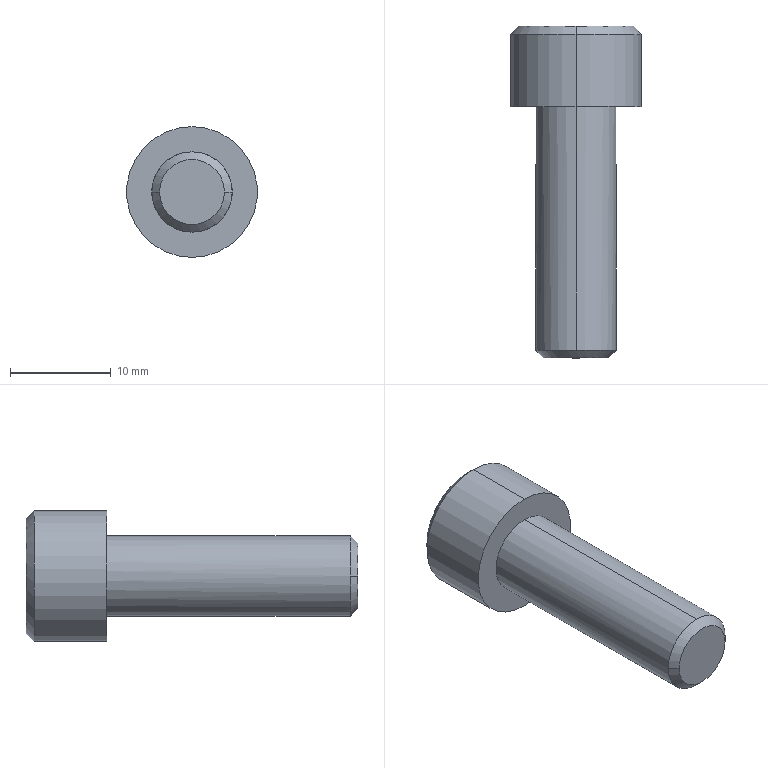Part | STEP file | PN59104-141_M_SHCSM8x1.25x25 | 1 solid | 18 faces | box 13 x 33 x 13 mm | volume 2174 mm3 | plane 10 | cylinder 4 | cone 4 | commonest cylinder face diameters 8 x2 13 x2
STEP:
#1=CARTESIAN_POINT('',(0.,0.,-4.));
#2=VERTEX_POINT('',#1);
#3=CARTESIAN_POINT('',(0.,0.,4.));
#4=VERTEX_POINT('',#3);
#5=CARTESIAN_POINT('',(0.,0.,0.));
#6=DIRECTION('',(0.,-1.,0.));
#7=DIRECTION('',(0.,0.,-1.));
#8=AXIS2_PLACEMENT_3D('',#5,#6,#7);
#9=CIRCLE('',#8,4.);
#10=EDGE_CURVE('',#2,#4,#9,.T.);
#11=ORIENTED_EDGE('',*,*,#10,.T.);
#12=CARTESIAN_POINT('',(0.,-24.233,4.));
#13=VERTEX_POINT('',#12);
#14=CARTESIAN_POINT('',(0.,-25.,4.));
#15=DIRECTION('',(0.,-1.,0.));
#16=VECTOR('',#15,1000.);
#17=LINE('',#14,#16);
#18=EDGE_CURVE('',#4,#13,#17,.T.);
#19=ORIENTED_EDGE('',*,*,#18,.T.);
#20=CARTESIAN_POINT('',(4.,-24.233,0.));
#21=VERTEX_POINT('',#20);
#22=CARTESIAN_POINT('',(0.,-24.233,0.));
#23=DIRECTION('',(0.,1.,0.));
#24=DIRECTION('',(0.,0.,-1.));
#25=AXIS2_PLACEMENT_3D('',#22,#23,#24);
#26=CIRCLE('',#25,4.);
#27=EDGE_CURVE('',#13,#21,#26,.T.);
#28=ORIENTED_EDGE('',*,*,#27,.T.);
#29=CARTESIAN_POINT('',(0.,-24.233,-4.));
#30=VERTEX_POINT('',#29);
#31=CARTESIAN_POINT('',(0.,-24.233,0.));
#32=DIRECTION('',(0.,1.,0.));
#33=DIRECTION('',(0.,0.,-1.));
#34=AXIS2_PLACEMENT_3D('',#31,#32,#33);
#35=CIRCLE('',#34,4.);
#36=EDGE_CURVE('',#21,#30,#35,.T.);
#37=ORIENTED_EDGE('',*,*,#36,.T.);
#38=CARTESIAN_POINT('',(0.,-25.,-4.));
#39=DIRECTION('',(0.,-1.,0.));
#40=VECTOR('',#39,1000.);
#41=LINE('',#38,#40);
#42=EDGE_CURVE('',#2,#30,#41,.T.);
#43=ORIENTED_EDGE('',*,*,#42,.F.);
#44=EDGE_LOOP('',(#11,#19,#28,#37,#43));
#45=FACE_OUTER_BOUND('',#44,.T.);
#46=CARTESIAN_POINT('',(0.,-25.,0.));
#47=DIRECTION('',(0.,-1.,0.));
#48=DIRECTION('',(0.,0.,-1.));
#49=AXIS2_PLACEMENT_3D('',#46,#47,#48);
#50=CYLINDRICAL_SURFACE('',#49,4.);
#51=ADVANCED_FACE('',(#45),#50,.T.);
#52=CARTESIAN_POINT('',(-3.233,-25.,0.));
#53=VERTEX_POINT('',#52);
#54=CARTESIAN_POINT('',(3.233,-25.,0.));
#55=VERTEX_POINT('',#54);
#56=CARTESIAN_POINT('',(0.,-25.,0.));
#57=DIRECTION('',(0.,1.,0.));
#58=DIRECTION('',(-1.,0.,0.));
#59=AXIS2_PLACEMENT_3D('',#56,#57,#58);
#60=CIRCLE('',#59,3.233);
#61=EDGE_CURVE('',#53,#55,#60,.T.);
#62=ORIENTED_EDGE('',*,*,#61,.T.);
#63=CARTESIAN_POINT('',(4.,-24.233,0.));
#64=DIRECTION('',(0.7071,0.7071,0.));
#65=VECTOR('',#64,1000.);
#66=LINE('',#63,#65);
#67=EDGE_CURVE('',#55,#21,#66,.T.);
#68=ORIENTED_EDGE('',*,*,#67,.T.);
#69=ORIENTED_EDGE('',*,*,#27,.F.);
#70=CARTESIAN_POINT('',(-4.,-24.233,0.));
#71=VERTEX_POINT('',#70);
#72=CARTESIAN_POINT('',(0.,-24.233,0.));
#73=DIRECTION('',(0.,1.,0.));
#74=DIRECTION('',(0.,0.,-1.));
#75=AXIS2_PLACEMENT_3D('',#72,#73,#74);
#76=CIRCLE('',#75,4.);
#77=EDGE_CURVE('',#71,#13,#76,.T.);
#78=ORIENTED_EDGE('',*,*,#77,.F.);
#79=CARTESIAN_POINT('',(-4.,-24.233,0.));
#80=DIRECTION('',(-0.7071,0.7071,0.));
#81=VECTOR('',#80,1000.);
#82=LINE('',#79,#81);
#83=EDGE_CURVE('',#53,#71,#82,.T.);
#84=ORIENTED_EDGE('',*,*,#83,.F.);
#85=EDGE_LOOP('',(#62,#68,#69,#78,#84));
#86=FACE_OUTER_BOUND('',#85,.T.);
#87=CARTESIAN_POINT('',(0.,-24.233,0.));
#88=DIRECTION('',(0.,1.,0.));
#89=DIRECTION('',(-1.,0.,0.));
#90=AXIS2_PLACEMENT_3D('',#87,#88,#89);
#91=CONICAL_SURFACE('',#90,4.,0.7854);
#92=ADVANCED_FACE('',(#86),#91,.T.);
#93=CARTESIAN_POINT('',(0.,7.2,-6.5));
#94=VERTEX_POINT('',#93);
#95=CARTESIAN_POINT('',(0.,7.2,6.5));
#96=VERTEX_POINT('',#95);
#97=CARTESIAN_POINT('',(0.,7.2,0.));
#98=DIRECTION('',(0.,-1.,0.));
#99=DIRECTION('',(0.,0.,-1.));
#100=AXIS2_PLACEMENT_3D('',#97,#98,#99);
#101=CIRCLE('',#100,6.5);
#102=EDGE_CURVE('',#94,#96,#101,.T.);
#103=ORIENTED_EDGE('',*,*,#102,.T.);
#104=CARTESIAN_POINT('',(0.,0.,6.5));
#105=VERTEX_POINT('',#104);
#106=CARTESIAN_POINT('',(0.,-25.,6.5));
#107=DIRECTION('',(0.,-1.,0.));
#108=VECTOR('',#107,1000.);
#109=LINE('',#106,#108);
#110=EDGE_CURVE('',#96,#105,#109,.T.);
#111=ORIENTED_EDGE('',*,*,#110,.T.);
#112=CARTESIAN_POINT('',(0.,0.,-6.5));
#113=VERTEX_POINT('',#112);
#114=CARTESIAN_POINT('',(0.,0.,0.));
#115=DIRECTION('',(0.,1.,0.));
#116=DIRECTION('',(0.,0.,-1.));
#117=AXIS2_PLACEMENT_3D('',#114,#115,#116);
#118=CIRCLE('',#117,6.5);
#119=EDGE_CURVE('',#105,#113,#118,.T.);
#120=ORIENTED_EDGE('',*,*,#119,.T.);
#121=CARTESIAN_POINT('',(0.,-25.,-6.5));
#122=DIRECTION('',(0.,-1.,0.));
#123=VECTOR('',#122,1000.);
#124=LINE('',#121,#123);
#125=EDGE_CURVE('',#94,#113,#124,.T.);
#126=ORIENTED_EDGE('',*,*,#125,.F.);
#127=EDGE_LOOP('',(#103,#111,#120,#126));
#128=FACE_OUTER_BOUND('',#127,.T.);
#129=CARTESIAN_POINT('',(0.,-25.,0.));
#130=DIRECTION('',(0.,-1.,0.));
#131=DIRECTION('',(0.,0.,-1.));
#132=AXIS2_PLACEMENT_3D('',#129,#130,#131);
#133=CYLINDRICAL_SURFACE('',#132,6.5);
#134=ADVANCED_FACE('',(#128),#133,.T.);
#135=CARTESIAN_POINT('',(0.,8.,-5.7));
#136=VERTEX_POINT('',#135);
#137=CARTESIAN_POINT('',(0.,8.,5.7));
#138=VERTEX_POINT('',#137);
#139=CARTESIAN_POINT('',(0.,8.,0.));
#140=DIRECTION('',(0.,-1.,0.));
#141=DIRECTION('',(0.,0.,-1.));
#142=AXIS2_PLACEMENT_3D('',#139,#140,#141);
#143=CIRCLE('',#142,5.7);
#144=EDGE_CURVE('',#136,#138,#143,.T.);
#145=ORIENTED_EDGE('',*,*,#144,.T.);
#146=CARTESIAN_POINT('',(0.,7.2,6.5));
#147=DIRECTION('',(0.,-0.7071,0.7071));
#148=VECTOR('',#147,1000.);
#149=LINE('',#146,#148);
#150=EDGE_CURVE('',#138,#96,#149,.T.);
#151=ORIENTED_EDGE('',*,*,#150,.T.);
#152=ORIENTED_EDGE('',*,*,#102,.F.);
#153=CARTESIAN_POINT('',(0.,7.2,-6.5));
#154=DIRECTION('',(0.,-0.7071,-0.7071));
#155=VECTOR('',#154,1000.);
#156=LINE('',#153,#155);
#157=EDGE_CURVE('',#136,#94,#156,.T.);
#158=ORIENTED_EDGE('',*,*,#157,.F.);
#159=EDGE_LOOP('',(#145,#151,#152,#158));
#160=FACE_OUTER_BOUND('',#159,.T.);
#161=CARTESIAN_POINT('',(0.,7.2,0.));
#162=DIRECTION('',(0.,-1.,0.));
#163=DIRECTION('',(0.,0.,-1.));
#164=AXIS2_PLACEMENT_3D('',#161,#162,#163);
#165=CONICAL_SURFACE('',#164,6.5,0.7854);
#166=ADVANCED_FACE('',(#160),#165,.T.);
#167=ORIENTED_EDGE('',*,*,#18,.F.);
#168=CARTESIAN_POINT('',(0.,0.,0.));
#169=DIRECTION('',(0.,-1.,0.));
#170=DIRECTION('',(0.,0.,-1.));
#171=AXIS2_PLACEMENT_3D('',#168,#169,#170);
#172=CIRCLE('',#171,4.);
#173=EDGE_CURVE('',#4,#2,#172,.T.);
#174=ORIENTED_EDGE('',*,*,#173,.T.);
#175=ORIENTED_EDGE('',*,*,#42,.T.);
#176=CARTESIAN_POINT('',(0.,-24.233,0.));
#177=DIRECTION('',(0.,1.,0.));
#178=DIRECTION('',(0.,0.,-1.));
#179=AXIS2_PLACEMENT_3D('',#176,#177,#178);
#180=CIRCLE('',#179,4.);
#181=EDGE_CURVE('',#30,#71,#180,.T.);
#182=ORIENTED_EDGE('',*,*,#181,.T.);
#183=ORIENTED_EDGE('',*,*,#77,.T.);
#184=EDGE_LOOP('',(#167,#174,#175,#182,#183));
#185=FACE_OUTER_BOUND('',#184,.T.);
#186=CARTESIAN_POINT('',(0.,-25.,0.));
#187=DIRECTION('',(0.,-1.,0.));
#188=DIRECTION('',(0.,0.,-1.));
#189=AXIS2_PLACEMENT_3D('',#186,#187,#188);
#190=CYLINDRICAL_SURFACE('',#189,4.);
#191=ADVANCED_FACE('',(#185),#190,.T.);
#192=CARTESIAN_POINT('',(0.,0.,0.));
#193=DIRECTION('',(0.,1.,0.));
#194=DIRECTION('',(0.,0.,-1.));
#195=AXIS2_PLACEMENT_3D('',#192,#193,#194);
#196=CIRCLE('',#195,6.5);
#197=EDGE_CURVE('',#113,#105,#196,.T.);
#198=ORIENTED_EDGE('',*,*,#197,.F.);
#199=ORIENTED_EDGE('',*,*,#119,.F.);
#200=EDGE_LOOP('',(#198,#199));
#201=FACE_OUTER_BOUND('',#200,.T.);
#202=ORIENTED_EDGE('',*,*,#10,.F.);
#203=ORIENTED_EDGE('',*,*,#173,.F.);
#204=EDGE_LOOP('',(#202,#203));
#205=FACE_BOUND('',#204,.T.);
#206=CARTESIAN_POINT('',(6.5,0.,0.));
#207=DIRECTION('',(0.,1.,0.));
#208=DIRECTION('',(0.,0.,1.));
#209=AXIS2_PLACEMENT_3D('',#206,#207,#208);
#210=PLANE('',#209);
#211=ADVANCED_FACE('',(#201,#205),#210,.F.);
#212=ORIENTED_EDGE('',*,*,#67,.F.);
#213=CARTESIAN_POINT('',(0.,-25.,0.));
#214=DIRECTION('',(0.,1.,0.));
#215=DIRECTION('',(-1.,0.,0.));
#216=AXIS2_PLACEMENT_3D('',#213,#214,#215);
#217=CIRCLE('',#216,3.233);
#218=EDGE_CURVE('',#55,#53,#217,.T.);
#219=ORIENTED_EDGE('',*,*,#218,.T.);
#220=ORIENTED_EDGE('',*,*,#83,.T.);
#221=ORIENTED_EDGE('',*,*,#181,.F.);
#222=ORIENTED_EDGE('',*,*,#36,.F.);
#223=EDGE_LOOP('',(#212,#219,#220,#221,#222));
#224=FACE_OUTER_BOUND('',#223,.T.);
#225=CARTESIAN_POINT('',(0.,-24.233,0.));
#226=DIRECTION('',(0.,1.,0.));
#227=DIRECTION('',(-1.,0.,0.));
#228=AXIS2_PLACEMENT_3D('',#225,#226,#227);
#229=CONICAL_SURFACE('',#228,4.,0.7854);
#230=ADVANCED_FACE('',(#224),#229,.T.);
#231=ORIENTED_EDGE('',*,*,#110,.F.);
#232=CARTESIAN_POINT('',(0.,7.2,0.));
#233=DIRECTION('',(0.,-1.,0.));
#234=DIRECTION('',(0.,0.,-1.));
#235=AXIS2_PLACEMENT_3D('',#232,#233,#234);
#236=CIRCLE('',#235,6.5);
#237=EDGE_CURVE('',#96,#94,#236,.T.);
#238=ORIENTED_EDGE('',*,*,#237,.T.);
#239=ORIENTED_EDGE('',*,*,#125,.T.);
#240=ORIENTED_EDGE('',*,*,#197,.T.);
#241=EDGE_LOOP('',(#231,#238,#239,#240));
#242=FACE_OUTER_BOUND('',#241,.T.);
#243=CARTESIAN_POINT('',(0.,-25.,0.));
#244=DIRECTION('',(0.,-1.,0.));
#245=DIRECTION('',(0.,0.,-1.));
#246=AXIS2_PLACEMENT_3D('',#243,#244,#245);
#247=CYLINDRICAL_SURFACE('',#246,6.5);
#248=ADVANCED_FACE('',(#242),#247,.T.);
#249=ORIENTED_EDGE('',*,*,#61,.F.);
#250=ORIENTED_EDGE('',*,*,#218,.F.);
#251=EDGE_LOOP('',(#249,#250));
#252=FACE_OUTER_BOUND('',#251,.T.);
#253=CARTESIAN_POINT('',(3.233,-25.,0.));
#254=DIRECTION('',(0.,1.,0.));
#255=DIRECTION('',(0.,0.,1.));
#256=AXIS2_PLACEMENT_3D('',#253,#254,#255);
#257=PLANE('',#256);
#258=ADVANCED_FACE('',(#252),#257,.F.);
#259=ORIENTED_EDGE('',*,*,#150,.F.);
#260=CARTESIAN_POINT('',(0.,8.,0.));
#261=DIRECTION('',(0.,-1.,0.));
#262=DIRECTION('',(0.,0.,-1.));
#263=AXIS2_PLACEMENT_3D('',#260,#261,#262);
#264=CIRCLE('',#263,5.7);
#265=EDGE_CURVE('',#138,#136,#264,.T.);
#266=ORIENTED_EDGE('',*,*,#265,.T.);
#267=ORIENTED_EDGE('',*,*,#157,.T.);
#268=ORIENTED_EDGE('',*,*,#237,.F.);
#269=EDGE_LOOP('',(#259,#266,#267,#268));
#270=FACE_OUTER_BOUND('',#269,.T.);
#271=CARTESIAN_POINT('',(0.,7.2,0.));
#272=DIRECTION('',(0.,-1.,0.));
#273=DIRECTION('',(0.,0.,-1.));
#274=AXIS2_PLACEMENT_3D('',#271,#272,#273);
#275=CONICAL_SURFACE('',#274,6.5,0.7854);
#276=ADVANCED_FACE('',(#270),#275,.T.);
#277=CARTESIAN_POINT('',(-3.,8.,1.732));
#278=VERTEX_POINT('',#277);
#279=CARTESIAN_POINT('',(0.,8.,3.464));
#280=VERTEX_POINT('',#279);
#281=CARTESIAN_POINT('',(-3.,8.,1.732));
#282=DIRECTION('',(0.866,0.,0.5));
#283=VECTOR('',#282,1000.);
#284=LINE('',#281,#283);
#285=EDGE_CURVE('',#278,#280,#284,.T.);
#286=ORIENTED_EDGE('',*,*,#285,.F.);
#287=CARTESIAN_POINT('',(-3.,8.,-1.732));
#288=VERTEX_POINT('',#287);
#289=CARTESIAN_POINT('',(-3.,8.,0.));
#290=DIRECTION('',(0.,0.,1.));
#291=VECTOR('',#290,1000.);
#292=LINE('',#289,#291);
#293=EDGE_CURVE('',#288,#278,#292,.T.);
#294=ORIENTED_EDGE('',*,*,#293,.F.);
#295=CARTESIAN_POINT('',(0.,8.,-3.464));
#296=VERTEX_POINT('',#295);
#297=CARTESIAN_POINT('',(0.,8.,-3.464));
#298=DIRECTION('',(-0.866,0.,0.5));
#299=VECTOR('',#298,1000.);
#300=LINE('',#297,#299);
#301=EDGE_CURVE('',#296,#288,#300,.T.);
#302=ORIENTED_EDGE('',*,*,#301,.F.);
#303=CARTESIAN_POINT('',(3.,8.,-1.732));
#304=VERTEX_POINT('',#303);
#305=CARTESIAN_POINT('',(3.,8.,-1.732));
#306=DIRECTION('',(-0.866,0.,-0.5));
#307=VECTOR('',#306,1000.);
#308=LINE('',#305,#307);
#309=EDGE_CURVE('',#304,#296,#308,.T.);
#310=ORIENTED_EDGE('',*,*,#309,.F.);
#311=CARTESIAN_POINT('',(3.,8.,1.732));
#312=VERTEX_POINT('',#311);
#313=CARTESIAN_POINT('',(3.,8.,0.));
#314=DIRECTION('',(0.,0.,-1.));
#315=VECTOR('',#314,1000.);
#316=LINE('',#313,#315);
#317=EDGE_CURVE('',#312,#304,#316,.T.);
#318=ORIENTED_EDGE('',*,*,#317,.F.);
#319=CARTESIAN_POINT('',(0.,8.,3.464));
#320=DIRECTION('',(0.866,0.,-0.5));
#321=VECTOR('',#320,1000.);
#322=LINE('',#319,#321);
#323=EDGE_CURVE('',#280,#312,#322,.T.);
#324=ORIENTED_EDGE('',*,*,#323,.F.);
#325=EDGE_LOOP('',(#286,#294,#302,#310,#318,#324));
#326=FACE_BOUND('',#325,.T.);
#327=ORIENTED_EDGE('',*,*,#144,.F.);
#328=ORIENTED_EDGE('',*,*,#265,.F.);
#329=EDGE_LOOP('',(#327,#328));
#330=FACE_OUTER_BOUND('',#329,.T.);
#331=CARTESIAN_POINT('',(0.,8.,0.));
#332=DIRECTION('',(0.,-1.,0.));
#333=DIRECTION('',(0.,0.,-1.));
#334=AXIS2_PLACEMENT_3D('',#331,#332,#333);
#335=PLANE('',#334);
#336=ADVANCED_FACE('',(#326,#330),#335,.F.);
#337=CARTESIAN_POINT('',(3.,4.,1.732));
#338=VERTEX_POINT('',#337);
#339=CARTESIAN_POINT('',(3.,4.,1.732));
#340=DIRECTION('',(0.,1.,0.));
#341=VECTOR('',#340,1000.);
#342=LINE('',#339,#341);
#343=EDGE_CURVE('',#338,#312,#342,.T.);
#344=ORIENTED_EDGE('',*,*,#343,.F.);
#345=CARTESIAN_POINT('',(0.,4.,3.464));
#346=VERTEX_POINT('',#345);
#347=CARTESIAN_POINT('',(0.,4.,3.464));
#348=DIRECTION('',(0.866,0.,-0.5));
#349=VECTOR('',#348,1000.);
#350=LINE('',#347,#349);
#351=EDGE_CURVE('',#346,#338,#350,.T.);
#352=ORIENTED_EDGE('',*,*,#351,.F.);
#353=CARTESIAN_POINT('',(0.,4.,3.464));
#354=DIRECTION('',(0.,-1.,0.));
#355=VECTOR('',#354,1000.);
#356=LINE('',#353,#355);
#357=EDGE_CURVE('',#280,#346,#356,.T.);
#358=ORIENTED_EDGE('',*,*,#357,.F.);
#359=ORIENTED_EDGE('',*,*,#323,.T.);
#360=EDGE_LOOP('',(#344,#352,#358,#359));
#361=FACE_OUTER_BOUND('',#360,.T.);
#362=CARTESIAN_POINT('',(0.,4.,3.464));
#363=DIRECTION('',(0.5,0.,0.866));
#364=DIRECTION('',(0.866,0.,-0.5));
#365=AXIS2_PLACEMENT_3D('',#362,#363,#364);
#366=PLANE('',#365);
#367=ADVANCED_FACE('',(#361),#366,.F.);
#368=ORIENTED_EDGE('',*,*,#357,.T.);
#369=CARTESIAN_POINT('',(-3.,4.,1.732));
#370=VERTEX_POINT('',#369);
#371=CARTESIAN_POINT('',(-3.,4.,1.732));
#372=DIRECTION('',(0.866,0.,0.5));
#373=VECTOR('',#372,1000.);
#374=LINE('',#371,#373);
#375=EDGE_CURVE('',#370,#346,#374,.T.);
#376=ORIENTED_EDGE('',*,*,#375,.F.);
#377=CARTESIAN_POINT('',(-3.,4.,1.732));
#378=DIRECTION('',(0.,-1.,0.));
#379=VECTOR('',#378,1000.);
#380=LINE('',#377,#379);
#381=EDGE_CURVE('',#278,#370,#380,.T.);
#382=ORIENTED_EDGE('',*,*,#381,.F.);
#383=ORIENTED_EDGE('',*,*,#285,.T.);
#384=EDGE_LOOP('',(#368,#376,#382,#383));
#385=FACE_OUTER_BOUND('',#384,.T.);
#386=CARTESIAN_POINT('',(-3.,4.,1.732));
#387=DIRECTION('',(-0.5,0.,0.866));
#388=DIRECTION('',(0.866,0.,0.5));
#389=AXIS2_PLACEMENT_3D('',#386,#387,#388);
#390=PLANE('',#389);
#391=ADVANCED_FACE('',(#385),#390,.F.);
#392=ORIENTED_EDGE('',*,*,#381,.T.);
#393=CARTESIAN_POINT('',(-3.,4.,-1.732));
#394=VERTEX_POINT('',#393);
#395=CARTESIAN_POINT('',(-3.,4.,-1.732));
#396=DIRECTION('',(0.,0.,1.));
#397=VECTOR('',#396,1000.);
#398=LINE('',#395,#397);
#399=EDGE_CURVE('',#394,#370,#398,.T.);
#400=ORIENTED_EDGE('',*,*,#399,.F.);
#401=CARTESIAN_POINT('',(-3.,4.,-1.732));
#402=DIRECTION('',(0.,-1.,0.));
#403=VECTOR('',#402,1000.);
#404=LINE('',#401,#403);
#405=EDGE_CURVE('',#288,#394,#404,.T.);
#406=ORIENTED_EDGE('',*,*,#405,.F.);
#407=ORIENTED_EDGE('',*,*,#293,.T.);
#408=EDGE_LOOP('',(#392,#400,#406,#407));
#409=FACE_OUTER_BOUND('',#408,.T.);
#410=CARTESIAN_POINT('',(-3.,4.,-1.732));
#411=DIRECTION('',(-1.,0.,0.));
#412=DIRECTION('',(0.,0.,1.));
#413=AXIS2_PLACEMENT_3D('',#410,#411,#412);
#414=PLANE('',#413);
#415=ADVANCED_FACE('',(#409),#414,.F.);
#416=ORIENTED_EDGE('',*,*,#405,.T.);
#417=CARTESIAN_POINT('',(0.,4.,-3.464));
#418=VERTEX_POINT('',#417);
#419=CARTESIAN_POINT('',(0.,4.,-3.464));
#420=DIRECTION('',(-0.866,0.,0.5));
#421=VECTOR('',#420,1000.);
#422=LINE('',#419,#421);
#423=EDGE_CURVE('',#418,#394,#422,.T.);
#424=ORIENTED_EDGE('',*,*,#423,.F.);
#425=CARTESIAN_POINT('',(0.,4.,-3.464));
#426=DIRECTION('',(0.,-1.,0.));
#427=VECTOR('',#426,1000.);
#428=LINE('',#425,#427);
#429=EDGE_CURVE('',#296,#418,#428,.T.);
#430=ORIENTED_EDGE('',*,*,#429,.F.);
#431=ORIENTED_EDGE('',*,*,#301,.T.);
#432=EDGE_LOOP('',(#416,#424,#430,#431));
#433=FACE_OUTER_BOUND('',#432,.T.);
#434=CARTESIAN_POINT('',(0.,4.,-3.464));
#435=DIRECTION('',(-0.5,0.,-0.866));
#436=DIRECTION('',(-0.866,0.,0.5));
#437=AXIS2_PLACEMENT_3D('',#434,#435,#436);
#438=PLANE('',#437);
#439=ADVANCED_FACE('',(#433),#438,.F.);
#440=ORIENTED_EDGE('',*,*,#429,.T.);
#441=CARTESIAN_POINT('',(3.,4.,-1.732));
#442=VERTEX_POINT('',#441);
#443=CARTESIAN_POINT('',(3.,4.,-1.732));
#444=DIRECTION('',(-0.866,0.,-0.5));
#445=VECTOR('',#444,1000.);
#446=LINE('',#443,#445);
#447=EDGE_CURVE('',#442,#418,#446,.T.);
#448=ORIENTED_EDGE('',*,*,#447,.F.);
#449=CARTESIAN_POINT('',(3.,4.,-1.732));
#450=DIRECTION('',(0.,-1.,0.));
#451=VECTOR('',#450,1000.);
#452=LINE('',#449,#451);
#453=EDGE_CURVE('',#304,#442,#452,.T.);
#454=ORIENTED_EDGE('',*,*,#453,.F.);
#455=ORIENTED_EDGE('',*,*,#309,.T.);
#456=EDGE_LOOP('',(#440,#448,#454,#455));
#457=FACE_OUTER_BOUND('',#456,.T.);
#458=CARTESIAN_POINT('',(3.,4.,-1.732));
#459=DIRECTION('',(0.5,0.,-0.866));
#460=DIRECTION('',(-0.866,0.,-0.5));
#461=AXIS2_PLACEMENT_3D('',#458,#459,#460);
#462=PLANE('',#461);
#463=ADVANCED_FACE('',(#457),#462,.F.);
#464=ORIENTED_EDGE('',*,*,#317,.T.);
#465=ORIENTED_EDGE('',*,*,#453,.T.);
#466=CARTESIAN_POINT('',(3.,4.,1.732));
#467=DIRECTION('',(0.,0.,-1.));
#468=VECTOR('',#467,1000.);
#469=LINE('',#466,#468);
#470=EDGE_CURVE('',#338,#442,#469,.T.);
#471=ORIENTED_EDGE('',*,*,#470,.F.);
#472=ORIENTED_EDGE('',*,*,#343,.T.);
#473=EDGE_LOOP('',(#464,#465,#471,#472));
#474=FACE_OUTER_BOUND('',#473,.T.);
#475=CARTESIAN_POINT('',(3.,4.,1.732));
#476=DIRECTION('',(1.,0.,0.));
#477=DIRECTION('',(0.,0.,-1.));
#478=AXIS2_PLACEMENT_3D('',#475,#476,#477);
#479=PLANE('',#478);
#480=ADVANCED_FACE('',(#474),#479,.F.);
#481=ORIENTED_EDGE('',*,*,#447,.T.);
#482=ORIENTED_EDGE('',*,*,#423,.T.);
#483=ORIENTED_EDGE('',*,*,#399,.T.);
#484=ORIENTED_EDGE('',*,*,#375,.T.);
#485=ORIENTED_EDGE('',*,*,#351,.T.);
#486=ORIENTED_EDGE('',*,*,#470,.T.);
#487=EDGE_LOOP('',(#481,#482,#483,#484,#485,#486));
#488=FACE_OUTER_BOUND('',#487,.T.);
#489=CARTESIAN_POINT('',(0.,4.,0.));
#490=DIRECTION('',(0.,1.,0.));
#491=DIRECTION('',(0.,0.,1.));
#492=AXIS2_PLACEMENT_3D('',#489,#490,#491);
#493=PLANE('',#492);
#494=ADVANCED_FACE('',(#488),#493,.T.);
#495=CLOSED_SHELL('',(#51,#92,#134,#166,#191,#211,#230,#248,#258,#276,#336,#367,#391,#415,#439,#463,#480,#494));
#496=MANIFOLD_SOLID_BREP('',#495);
#497=CARTESIAN_POINT('',(0.,0.,0.));
#498=DIRECTION('',(0.,0.,1.));
#499=DIRECTION('',(1.,0.,0.));
#500=AXIS2_PLACEMENT_3D('',#497,#498,#499);
#501=(LENGTH_UNIT()NAMED_UNIT(*)SI_UNIT(.MILLI.,.METRE.));
#502=UNCERTAINTY_MEASURE_WITH_UNIT(LENGTH_MEASURE(0.00001),#501,'','');
#503=(NAMED_UNIT(*)PLANE_ANGLE_UNIT()SI_UNIT($,.RADIAN.));
#504=(NAMED_UNIT(*)SI_UNIT($,.STERADIAN.)SOLID_ANGLE_UNIT());
#505=(GEOMETRIC_REPRESENTATION_CONTEXT(3)GLOBAL_UNCERTAINTY_ASSIGNED_CONTEXT((#502))GLOBAL_UNIT_ASSIGNED_CONTEXT((#501,#503,#504))REPRESENTATION_CONTEXT('',''));
#506=ADVANCED_BREP_SHAPE_REPRESENTATION('',(#496,#500),#505);